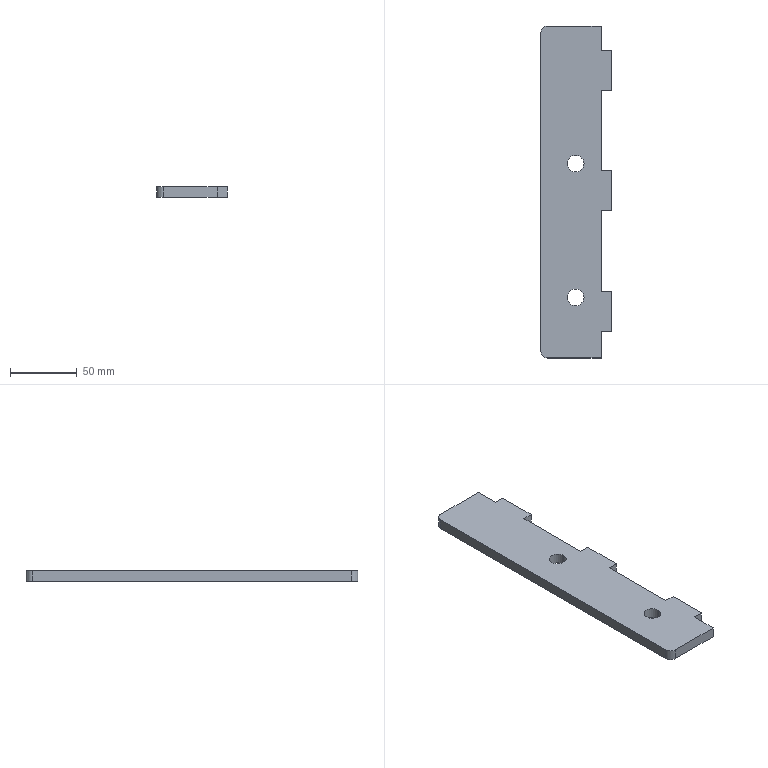Part | SolidWorks | features FlatPattern 1, SMBaseFlange 1, SheetMetal 1 | 1 solid | 24 faces | box 52.5 x 248 x 8 mm | volume 92631 mm3 | plane 18 | cylinder 6 | commonest cylinder face diameters 12.5 x4 10 x2
STEP:
#1=CARTESIAN_POINT('',(-25.25,44.,8.));
#2=VERTEX_POINT('',#1);
#3=CARTESIAN_POINT('',(-12.75,44.,8.));
#4=VERTEX_POINT('',#3);
#5=CARTESIAN_POINT('',(-19.,44.,8.));
#6=DIRECTION('',(0.,0.,1.));
#7=DIRECTION('',(1.,0.,0.));
#8=AXIS2_PLACEMENT_3D('',#5,#6,#7);
#9=CIRCLE('',#8,6.25);
#10=EDGE_CURVE('',#2,#4,#9,.T.);
#11=ORIENTED_EDGE('',*,*,#10,.T.);
#12=CARTESIAN_POINT('',(-12.75,44.,0.));
#13=VERTEX_POINT('',#12);
#14=CARTESIAN_POINT('',(-12.75,44.,8.));
#15=DIRECTION('',(0.,0.,-1.));
#16=VECTOR('',#15,1000.);
#17=LINE('',#14,#16);
#18=EDGE_CURVE('',#4,#13,#17,.T.);
#19=ORIENTED_EDGE('',*,*,#18,.T.);
#20=CARTESIAN_POINT('',(-25.25,44.,0.));
#21=VERTEX_POINT('',#20);
#22=CARTESIAN_POINT('',(-19.,44.,0.));
#23=DIRECTION('',(0.,0.,1.));
#24=DIRECTION('',(1.,0.,0.));
#25=AXIS2_PLACEMENT_3D('',#22,#23,#24);
#26=CIRCLE('',#25,6.25);
#27=EDGE_CURVE('',#21,#13,#26,.T.);
#28=ORIENTED_EDGE('',*,*,#27,.F.);
#29=CARTESIAN_POINT('',(-25.25,44.,8.));
#30=DIRECTION('',(0.,0.,-1.));
#31=VECTOR('',#30,1000.);
#32=LINE('',#29,#31);
#33=EDGE_CURVE('',#2,#21,#32,.T.);
#34=ORIENTED_EDGE('',*,*,#33,.F.);
#35=EDGE_LOOP('',(#11,#19,#28,#34));
#36=FACE_OUTER_BOUND('',#35,.T.);
#37=CARTESIAN_POINT('',(-19.,44.,8.));
#38=DIRECTION('',(0.,0.,-1.));
#39=DIRECTION('',(-1.,0.,0.));
#40=AXIS2_PLACEMENT_3D('',#37,#38,#39);
#41=CYLINDRICAL_SURFACE('',#40,6.25);
#42=ADVANCED_FACE('',(#36),#41,.F.);
#43=CARTESIAN_POINT('',(-25.25,-56.,8.));
#44=VERTEX_POINT('',#43);
#45=CARTESIAN_POINT('',(-12.75,-56.,8.));
#46=VERTEX_POINT('',#45);
#47=CARTESIAN_POINT('',(-19.,-56.,8.));
#48=DIRECTION('',(0.,0.,1.));
#49=DIRECTION('',(1.,0.,0.));
#50=AXIS2_PLACEMENT_3D('',#47,#48,#49);
#51=CIRCLE('',#50,6.25);
#52=EDGE_CURVE('',#44,#46,#51,.T.);
#53=ORIENTED_EDGE('',*,*,#52,.T.);
#54=CARTESIAN_POINT('',(-12.75,-56.,0.));
#55=VERTEX_POINT('',#54);
#56=CARTESIAN_POINT('',(-12.75,-56.,8.));
#57=DIRECTION('',(0.,0.,-1.));
#58=VECTOR('',#57,1000.);
#59=LINE('',#56,#58);
#60=EDGE_CURVE('',#46,#55,#59,.T.);
#61=ORIENTED_EDGE('',*,*,#60,.T.);
#62=CARTESIAN_POINT('',(-25.25,-56.,0.));
#63=VERTEX_POINT('',#62);
#64=CARTESIAN_POINT('',(-19.,-56.,0.));
#65=DIRECTION('',(0.,0.,1.));
#66=DIRECTION('',(1.,0.,0.));
#67=AXIS2_PLACEMENT_3D('',#64,#65,#66);
#68=CIRCLE('',#67,6.25);
#69=EDGE_CURVE('',#63,#55,#68,.T.);
#70=ORIENTED_EDGE('',*,*,#69,.F.);
#71=CARTESIAN_POINT('',(-25.25,-56.,8.));
#72=DIRECTION('',(0.,0.,-1.));
#73=VECTOR('',#72,1000.);
#74=LINE('',#71,#73);
#75=EDGE_CURVE('',#44,#63,#74,.T.);
#76=ORIENTED_EDGE('',*,*,#75,.F.);
#77=EDGE_LOOP('',(#53,#61,#70,#76));
#78=FACE_OUTER_BOUND('',#77,.T.);
#79=CARTESIAN_POINT('',(-19.,-56.,8.));
#80=DIRECTION('',(0.,0.,-1.));
#81=DIRECTION('',(-1.,0.,0.));
#82=AXIS2_PLACEMENT_3D('',#79,#80,#81);
#83=CYLINDRICAL_SURFACE('',#82,6.25);
#84=ADVANCED_FACE('',(#78),#83,.F.);
#85=CARTESIAN_POINT('',(0.,-101.22,8.));
#86=VERTEX_POINT('',#85);
#87=CARTESIAN_POINT('',(0.,-81.22,8.));
#88=VERTEX_POINT('',#87);
#89=CARTESIAN_POINT('',(0.,-101.22,8.));
#90=DIRECTION('',(0.,1.,0.));
#91=VECTOR('',#90,1000.);
#92=LINE('',#89,#91);
#93=EDGE_CURVE('',#86,#88,#92,.T.);
#94=ORIENTED_EDGE('',*,*,#93,.T.);
#95=CARTESIAN_POINT('',(7.5,-81.22,8.));
#96=VERTEX_POINT('',#95);
#97=CARTESIAN_POINT('',(0.,-81.22,8.));
#98=DIRECTION('',(1.,0.,0.));
#99=VECTOR('',#98,1000.);
#100=LINE('',#97,#99);
#101=EDGE_CURVE('',#88,#96,#100,.T.);
#102=ORIENTED_EDGE('',*,*,#101,.T.);
#103=CARTESIAN_POINT('',(7.5,-51.22,8.));
#104=VERTEX_POINT('',#103);
#105=CARTESIAN_POINT('',(7.5,-81.22,8.));
#106=DIRECTION('',(0.,1.,0.));
#107=VECTOR('',#106,1000.);
#108=LINE('',#105,#107);
#109=EDGE_CURVE('',#96,#104,#108,.T.);
#110=ORIENTED_EDGE('',*,*,#109,.T.);
#111=CARTESIAN_POINT('',(0.,-51.22,8.));
#112=VERTEX_POINT('',#111);
#113=CARTESIAN_POINT('',(7.5,-51.22,8.));
#114=DIRECTION('',(-1.,0.,0.));
#115=VECTOR('',#114,1000.);
#116=LINE('',#113,#115);
#117=EDGE_CURVE('',#104,#112,#116,.T.);
#118=ORIENTED_EDGE('',*,*,#117,.T.);
#119=CARTESIAN_POINT('',(0.,8.78,8.));
#120=VERTEX_POINT('',#119);
#121=CARTESIAN_POINT('',(0.,8.78,8.));
#122=DIRECTION('',(0.,1.,0.));
#123=VECTOR('',#122,1000.);
#124=LINE('',#121,#123);
#125=EDGE_CURVE('',#112,#120,#124,.T.);
#126=ORIENTED_EDGE('',*,*,#125,.T.);
#127=CARTESIAN_POINT('',(7.5,8.78,8.));
#128=VERTEX_POINT('',#127);
#129=CARTESIAN_POINT('',(0.,8.78,8.));
#130=DIRECTION('',(1.,0.,0.));
#131=VECTOR('',#130,1000.);
#132=LINE('',#129,#131);
#133=EDGE_CURVE('',#120,#128,#132,.T.);
#134=ORIENTED_EDGE('',*,*,#133,.T.);
#135=CARTESIAN_POINT('',(7.5,38.78,8.));
#136=VERTEX_POINT('',#135);
#137=CARTESIAN_POINT('',(7.5,8.78,8.));
#138=DIRECTION('',(0.,1.,0.));
#139=VECTOR('',#138,1000.);
#140=LINE('',#137,#139);
#141=EDGE_CURVE('',#128,#136,#140,.T.);
#142=ORIENTED_EDGE('',*,*,#141,.T.);
#143=CARTESIAN_POINT('',(0.,38.78,8.));
#144=VERTEX_POINT('',#143);
#145=CARTESIAN_POINT('',(7.5,38.78,8.));
#146=DIRECTION('',(-1.,0.,0.));
#147=VECTOR('',#146,1000.);
#148=LINE('',#145,#147);
#149=EDGE_CURVE('',#136,#144,#148,.T.);
#150=ORIENTED_EDGE('',*,*,#149,.T.);
#151=CARTESIAN_POINT('',(0.,98.78,8.));
#152=VERTEX_POINT('',#151);
#153=CARTESIAN_POINT('',(0.,98.78,8.));
#154=DIRECTION('',(0.,1.,0.));
#155=VECTOR('',#154,1000.);
#156=LINE('',#153,#155);
#157=EDGE_CURVE('',#144,#152,#156,.T.);
#158=ORIENTED_EDGE('',*,*,#157,.T.);
#159=CARTESIAN_POINT('',(7.5,98.78,8.));
#160=VERTEX_POINT('',#159);
#161=CARTESIAN_POINT('',(0.,98.78,8.));
#162=DIRECTION('',(1.,0.,0.));
#163=VECTOR('',#162,1000.);
#164=LINE('',#161,#163);
#165=EDGE_CURVE('',#152,#160,#164,.T.);
#166=ORIENTED_EDGE('',*,*,#165,.T.);
#167=CARTESIAN_POINT('',(7.5,128.78,8.));
#168=VERTEX_POINT('',#167);
#169=CARTESIAN_POINT('',(7.5,98.78,8.));
#170=DIRECTION('',(0.,1.,0.));
#171=VECTOR('',#170,1000.);
#172=LINE('',#169,#171);
#173=EDGE_CURVE('',#160,#168,#172,.T.);
#174=ORIENTED_EDGE('',*,*,#173,.T.);
#175=CARTESIAN_POINT('',(0.,128.78,8.));
#176=VERTEX_POINT('',#175);
#177=CARTESIAN_POINT('',(7.5,128.78,8.));
#178=DIRECTION('',(-1.,0.,0.));
#179=VECTOR('',#178,1000.);
#180=LINE('',#177,#179);
#181=EDGE_CURVE('',#168,#176,#180,.T.);
#182=ORIENTED_EDGE('',*,*,#181,.T.);
#183=CARTESIAN_POINT('',(0.,146.78,8.));
#184=VERTEX_POINT('',#183);
#185=CARTESIAN_POINT('',(0.,146.78,8.));
#186=DIRECTION('',(0.,1.,0.));
#187=VECTOR('',#186,1000.);
#188=LINE('',#185,#187);
#189=EDGE_CURVE('',#176,#184,#188,.T.);
#190=ORIENTED_EDGE('',*,*,#189,.T.);
#191=CARTESIAN_POINT('',(-40.,146.78,8.));
#192=VERTEX_POINT('',#191);
#193=CARTESIAN_POINT('',(-40.,146.78,8.));
#194=DIRECTION('',(-1.,0.,0.));
#195=VECTOR('',#194,1000.);
#196=LINE('',#193,#195);
#197=EDGE_CURVE('',#184,#192,#196,.T.);
#198=ORIENTED_EDGE('',*,*,#197,.T.);
#199=CARTESIAN_POINT('',(-45.,141.78,8.));
#200=VERTEX_POINT('',#199);
#201=CARTESIAN_POINT('',(-40.,141.78,8.));
#202=DIRECTION('',(0.,0.,1.));
#203=DIRECTION('',(-1.,0.,0.));
#204=AXIS2_PLACEMENT_3D('',#201,#202,#203);
#205=CIRCLE('',#204,5.);
#206=EDGE_CURVE('',#192,#200,#205,.T.);
#207=ORIENTED_EDGE('',*,*,#206,.T.);
#208=CARTESIAN_POINT('',(-45.,-96.22,8.));
#209=VERTEX_POINT('',#208);
#210=CARTESIAN_POINT('',(-45.,-96.22,8.));
#211=DIRECTION('',(0.,-1.,0.));
#212=VECTOR('',#211,1000.);
#213=LINE('',#210,#212);
#214=EDGE_CURVE('',#200,#209,#213,.T.);
#215=ORIENTED_EDGE('',*,*,#214,.T.);
#216=CARTESIAN_POINT('',(-40.,-101.22,8.));
#217=VERTEX_POINT('',#216);
#218=CARTESIAN_POINT('',(-40.,-96.22,8.));
#219=DIRECTION('',(0.,0.,1.));
#220=DIRECTION('',(-1.,0.,0.));
#221=AXIS2_PLACEMENT_3D('',#218,#219,#220);
#222=CIRCLE('',#221,5.);
#223=EDGE_CURVE('',#209,#217,#222,.T.);
#224=ORIENTED_EDGE('',*,*,#223,.T.);
#225=CARTESIAN_POINT('',(0.,-101.22,8.));
#226=DIRECTION('',(1.,0.,0.));
#227=VECTOR('',#226,1000.);
#228=LINE('',#225,#227);
#229=EDGE_CURVE('',#217,#86,#228,.T.);
#230=ORIENTED_EDGE('',*,*,#229,.T.);
#231=EDGE_LOOP('',(#94,#102,#110,#118,#126,#134,#142,#150,#158,#166,#174,#182,#190,#198,#207,#215,#224,#230));
#232=FACE_OUTER_BOUND('',#231,.T.);
#233=ORIENTED_EDGE('',*,*,#52,.F.);
#234=CARTESIAN_POINT('',(-19.,-56.,8.));
#235=DIRECTION('',(0.,0.,1.));
#236=DIRECTION('',(1.,0.,0.));
#237=AXIS2_PLACEMENT_3D('',#234,#235,#236);
#238=CIRCLE('',#237,6.25);
#239=EDGE_CURVE('',#46,#44,#238,.T.);
#240=ORIENTED_EDGE('',*,*,#239,.F.);
#241=EDGE_LOOP('',(#233,#240));
#242=FACE_BOUND('',#241,.T.);
#243=ORIENTED_EDGE('',*,*,#10,.F.);
#244=CARTESIAN_POINT('',(-19.,44.,8.));
#245=DIRECTION('',(0.,0.,1.));
#246=DIRECTION('',(1.,0.,0.));
#247=AXIS2_PLACEMENT_3D('',#244,#245,#246);
#248=CIRCLE('',#247,6.25);
#249=EDGE_CURVE('',#4,#2,#248,.T.);
#250=ORIENTED_EDGE('',*,*,#249,.F.);
#251=EDGE_LOOP('',(#243,#250));
#252=FACE_BOUND('',#251,.T.);
#253=CARTESIAN_POINT('',(-40.,141.78,8.));
#254=DIRECTION('',(0.,0.,-1.));
#255=DIRECTION('',(-1.,0.,0.));
#256=AXIS2_PLACEMENT_3D('',#253,#254,#255);
#257=PLANE('',#256);
#258=ADVANCED_FACE('',(#232,#242,#252),#257,.F.);
#259=ORIENTED_EDGE('',*,*,#69,.T.);
#260=CARTESIAN_POINT('',(-19.,-56.,0.));
#261=DIRECTION('',(0.,0.,1.));
#262=DIRECTION('',(1.,0.,0.));
#263=AXIS2_PLACEMENT_3D('',#260,#261,#262);
#264=CIRCLE('',#263,6.25);
#265=EDGE_CURVE('',#55,#63,#264,.T.);
#266=ORIENTED_EDGE('',*,*,#265,.T.);
#267=EDGE_LOOP('',(#259,#266));
#268=FACE_BOUND('',#267,.T.);
#269=CARTESIAN_POINT('',(0.,-101.22,0.));
#270=VERTEX_POINT('',#269);
#271=CARTESIAN_POINT('',(0.,-81.22,0.));
#272=VERTEX_POINT('',#271);
#273=CARTESIAN_POINT('',(0.,-101.22,0.));
#274=DIRECTION('',(0.,1.,0.));
#275=VECTOR('',#274,1000.);
#276=LINE('',#273,#275);
#277=EDGE_CURVE('',#270,#272,#276,.T.);
#278=ORIENTED_EDGE('',*,*,#277,.F.);
#279=CARTESIAN_POINT('',(-40.,-101.22,0.));
#280=VERTEX_POINT('',#279);
#281=CARTESIAN_POINT('',(0.,-101.22,0.));
#282=DIRECTION('',(1.,0.,0.));
#283=VECTOR('',#282,1000.);
#284=LINE('',#281,#283);
#285=EDGE_CURVE('',#280,#270,#284,.T.);
#286=ORIENTED_EDGE('',*,*,#285,.F.);
#287=CARTESIAN_POINT('',(-45.,-96.22,0.));
#288=VERTEX_POINT('',#287);
#289=CARTESIAN_POINT('',(-40.,-96.22,0.));
#290=DIRECTION('',(0.,0.,1.));
#291=DIRECTION('',(-1.,0.,0.));
#292=AXIS2_PLACEMENT_3D('',#289,#290,#291);
#293=CIRCLE('',#292,5.);
#294=EDGE_CURVE('',#288,#280,#293,.T.);
#295=ORIENTED_EDGE('',*,*,#294,.F.);
#296=CARTESIAN_POINT('',(-45.,141.78,0.));
#297=VERTEX_POINT('',#296);
#298=CARTESIAN_POINT('',(-45.,-96.22,0.));
#299=DIRECTION('',(0.,-1.,0.));
#300=VECTOR('',#299,1000.);
#301=LINE('',#298,#300);
#302=EDGE_CURVE('',#297,#288,#301,.T.);
#303=ORIENTED_EDGE('',*,*,#302,.F.);
#304=CARTESIAN_POINT('',(-40.,146.78,0.));
#305=VERTEX_POINT('',#304);
#306=CARTESIAN_POINT('',(-40.,141.78,0.));
#307=DIRECTION('',(0.,0.,1.));
#308=DIRECTION('',(-1.,0.,0.));
#309=AXIS2_PLACEMENT_3D('',#306,#307,#308);
#310=CIRCLE('',#309,5.);
#311=EDGE_CURVE('',#305,#297,#310,.T.);
#312=ORIENTED_EDGE('',*,*,#311,.F.);
#313=CARTESIAN_POINT('',(0.,146.78,0.));
#314=VERTEX_POINT('',#313);
#315=CARTESIAN_POINT('',(-40.,146.78,0.));
#316=DIRECTION('',(-1.,0.,0.));
#317=VECTOR('',#316,1000.);
#318=LINE('',#315,#317);
#319=EDGE_CURVE('',#314,#305,#318,.T.);
#320=ORIENTED_EDGE('',*,*,#319,.F.);
#321=CARTESIAN_POINT('',(0.,128.78,0.));
#322=VERTEX_POINT('',#321);
#323=CARTESIAN_POINT('',(0.,146.78,0.));
#324=DIRECTION('',(0.,1.,0.));
#325=VECTOR('',#324,1000.);
#326=LINE('',#323,#325);
#327=EDGE_CURVE('',#322,#314,#326,.T.);
#328=ORIENTED_EDGE('',*,*,#327,.F.);
#329=CARTESIAN_POINT('',(7.5,128.78,0.));
#330=VERTEX_POINT('',#329);
#331=CARTESIAN_POINT('',(7.5,128.78,0.));
#332=DIRECTION('',(-1.,0.,0.));
#333=VECTOR('',#332,1000.);
#334=LINE('',#331,#333);
#335=EDGE_CURVE('',#330,#322,#334,.T.);
#336=ORIENTED_EDGE('',*,*,#335,.F.);
#337=CARTESIAN_POINT('',(7.5,98.78,0.));
#338=VERTEX_POINT('',#337);
#339=CARTESIAN_POINT('',(7.5,98.78,0.));
#340=DIRECTION('',(0.,1.,0.));
#341=VECTOR('',#340,1000.);
#342=LINE('',#339,#341);
#343=EDGE_CURVE('',#338,#330,#342,.T.);
#344=ORIENTED_EDGE('',*,*,#343,.F.);
#345=CARTESIAN_POINT('',(0.,98.78,0.));
#346=VERTEX_POINT('',#345);
#347=CARTESIAN_POINT('',(0.,98.78,0.));
#348=DIRECTION('',(1.,0.,0.));
#349=VECTOR('',#348,1000.);
#350=LINE('',#347,#349);
#351=EDGE_CURVE('',#346,#338,#350,.T.);
#352=ORIENTED_EDGE('',*,*,#351,.F.);
#353=CARTESIAN_POINT('',(0.,38.78,0.));
#354=VERTEX_POINT('',#353);
#355=CARTESIAN_POINT('',(0.,98.78,0.));
#356=DIRECTION('',(0.,1.,0.));
#357=VECTOR('',#356,1000.);
#358=LINE('',#355,#357);
#359=EDGE_CURVE('',#354,#346,#358,.T.);
#360=ORIENTED_EDGE('',*,*,#359,.F.);
#361=CARTESIAN_POINT('',(7.5,38.78,0.));
#362=VERTEX_POINT('',#361);
#363=CARTESIAN_POINT('',(7.5,38.78,0.));
#364=DIRECTION('',(-1.,0.,0.));
#365=VECTOR('',#364,1000.);
#366=LINE('',#363,#365);
#367=EDGE_CURVE('',#362,#354,#366,.T.);
#368=ORIENTED_EDGE('',*,*,#367,.F.);
#369=CARTESIAN_POINT('',(7.5,8.78,0.));
#370=VERTEX_POINT('',#369);
#371=CARTESIAN_POINT('',(7.5,8.78,0.));
#372=DIRECTION('',(0.,1.,0.));
#373=VECTOR('',#372,1000.);
#374=LINE('',#371,#373);
#375=EDGE_CURVE('',#370,#362,#374,.T.);
#376=ORIENTED_EDGE('',*,*,#375,.F.);
#377=CARTESIAN_POINT('',(0.,8.78,0.));
#378=VERTEX_POINT('',#377);
#379=CARTESIAN_POINT('',(0.,8.78,0.));
#380=DIRECTION('',(1.,0.,0.));
#381=VECTOR('',#380,1000.);
#382=LINE('',#379,#381);
#383=EDGE_CURVE('',#378,#370,#382,.T.);
#384=ORIENTED_EDGE('',*,*,#383,.F.);
#385=CARTESIAN_POINT('',(0.,-51.22,0.));
#386=VERTEX_POINT('',#385);
#387=CARTESIAN_POINT('',(0.,8.78,0.));
#388=DIRECTION('',(0.,1.,0.));
#389=VECTOR('',#388,1000.);
#390=LINE('',#387,#389);
#391=EDGE_CURVE('',#386,#378,#390,.T.);
#392=ORIENTED_EDGE('',*,*,#391,.F.);
#393=CARTESIAN_POINT('',(7.5,-51.22,0.));
#394=VERTEX_POINT('',#393);
#395=CARTESIAN_POINT('',(7.5,-51.22,0.));
#396=DIRECTION('',(-1.,0.,0.));
#397=VECTOR('',#396,1000.);
#398=LINE('',#395,#397);
#399=EDGE_CURVE('',#394,#386,#398,.T.);
#400=ORIENTED_EDGE('',*,*,#399,.F.);
#401=CARTESIAN_POINT('',(7.5,-81.22,0.));
#402=VERTEX_POINT('',#401);
#403=CARTESIAN_POINT('',(7.5,-81.22,0.));
#404=DIRECTION('',(0.,1.,0.));
#405=VECTOR('',#404,1000.);
#406=LINE('',#403,#405);
#407=EDGE_CURVE('',#402,#394,#406,.T.);
#408=ORIENTED_EDGE('',*,*,#407,.F.);
#409=CARTESIAN_POINT('',(0.,-81.22,0.));
#410=DIRECTION('',(1.,0.,0.));
#411=VECTOR('',#410,1000.);
#412=LINE('',#409,#411);
#413=EDGE_CURVE('',#272,#402,#412,.T.);
#414=ORIENTED_EDGE('',*,*,#413,.F.);
#415=EDGE_LOOP('',(#278,#286,#295,#303,#312,#320,#328,#336,#344,#352,#360,#368,#376,#384,#392,#400,#408,#414));
#416=FACE_OUTER_BOUND('',#415,.T.);
#417=ORIENTED_EDGE('',*,*,#27,.T.);
#418=CARTESIAN_POINT('',(-19.,44.,0.));
#419=DIRECTION('',(0.,0.,1.));
#420=DIRECTION('',(1.,0.,0.));
#421=AXIS2_PLACEMENT_3D('',#418,#419,#420);
#422=CIRCLE('',#421,6.25);
#423=EDGE_CURVE('',#13,#21,#422,.T.);
#424=ORIENTED_EDGE('',*,*,#423,.T.);
#425=EDGE_LOOP('',(#417,#424));
#426=FACE_BOUND('',#425,.T.);
#427=CARTESIAN_POINT('',(-40.,141.78,0.));
#428=DIRECTION('',(0.,0.,-1.));
#429=DIRECTION('',(-1.,0.,0.));
#430=AXIS2_PLACEMENT_3D('',#427,#428,#429);
#431=PLANE('',#430);
#432=ADVANCED_FACE('',(#268,#416,#426),#431,.T.);
#433=ORIENTED_EDGE('',*,*,#277,.T.);
#434=CARTESIAN_POINT('',(0.,-81.22,8.));
#435=DIRECTION('',(0.,0.,-1.));
#436=VECTOR('',#435,1000.);
#437=LINE('',#434,#436);
#438=EDGE_CURVE('',#88,#272,#437,.T.);
#439=ORIENTED_EDGE('',*,*,#438,.F.);
#440=ORIENTED_EDGE('',*,*,#93,.F.);
#441=CARTESIAN_POINT('',(0.,-101.22,8.));
#442=DIRECTION('',(0.,0.,-1.));
#443=VECTOR('',#442,1000.);
#444=LINE('',#441,#443);
#445=EDGE_CURVE('',#86,#270,#444,.T.);
#446=ORIENTED_EDGE('',*,*,#445,.T.);
#447=EDGE_LOOP('',(#433,#439,#440,#446));
#448=FACE_OUTER_BOUND('',#447,.T.);
#449=CARTESIAN_POINT('',(0.,-101.22,8.));
#450=DIRECTION('',(-1.,0.,0.));
#451=DIRECTION('',(0.,-1.,0.));
#452=AXIS2_PLACEMENT_3D('',#449,#450,#451);
#453=PLANE('',#452);
#454=ADVANCED_FACE('',(#448),#453,.F.);
#455=ORIENTED_EDGE('',*,*,#413,.T.);
#456=CARTESIAN_POINT('',(7.5,-81.22,8.));
#457=DIRECTION('',(0.,0.,-1.));
#458=VECTOR('',#457,1000.);
#459=LINE('',#456,#458);
#460=EDGE_CURVE('',#96,#402,#459,.T.);
#461=ORIENTED_EDGE('',*,*,#460,.F.);
#462=ORIENTED_EDGE('',*,*,#101,.F.);
#463=ORIENTED_EDGE('',*,*,#438,.T.);
#464=EDGE_LOOP('',(#455,#461,#462,#463));
#465=FACE_OUTER_BOUND('',#464,.T.);
#466=CARTESIAN_POINT('',(0.,-81.22,8.));
#467=DIRECTION('',(0.,1.,0.));
#468=DIRECTION('',(0.,0.,1.));
#469=AXIS2_PLACEMENT_3D('',#466,#467,#468);
#470=PLANE('',#469);
#471=ADVANCED_FACE('',(#465),#470,.F.);
#472=ORIENTED_EDGE('',*,*,#407,.T.);
#473=CARTESIAN_POINT('',(7.5,-51.22,8.));
#474=DIRECTION('',(0.,0.,-1.));
#475=VECTOR('',#474,1000.);
#476=LINE('',#473,#475);
#477=EDGE_CURVE('',#104,#394,#476,.T.);
#478=ORIENTED_EDGE('',*,*,#477,.F.);
#479=ORIENTED_EDGE('',*,*,#109,.F.);
#480=ORIENTED_EDGE('',*,*,#460,.T.);
#481=EDGE_LOOP('',(#472,#478,#479,#480));
#482=FACE_OUTER_BOUND('',#481,.T.);
#483=CARTESIAN_POINT('',(7.5,-81.22,8.));
#484=DIRECTION('',(-1.,0.,0.));
#485=DIRECTION('',(0.,0.,1.));
#486=AXIS2_PLACEMENT_3D('',#483,#484,#485);
#487=PLANE('',#486);
#488=ADVANCED_FACE('',(#482),#487,.F.);
#489=ORIENTED_EDGE('',*,*,#399,.T.);
#490=CARTESIAN_POINT('',(0.,-51.22,8.));
#491=DIRECTION('',(0.,0.,-1.));
#492=VECTOR('',#491,1000.);
#493=LINE('',#490,#492);
#494=EDGE_CURVE('',#112,#386,#493,.T.);
#495=ORIENTED_EDGE('',*,*,#494,.F.);
#496=ORIENTED_EDGE('',*,*,#117,.F.);
#497=ORIENTED_EDGE('',*,*,#477,.T.);
#498=EDGE_LOOP('',(#489,#495,#496,#497));
#499=FACE_OUTER_BOUND('',#498,.T.);
#500=CARTESIAN_POINT('',(7.5,-51.22,8.));
#501=DIRECTION('',(0.,-1.,0.));
#502=DIRECTION('',(0.,0.,-1.));
#503=AXIS2_PLACEMENT_3D('',#500,#501,#502);
#504=PLANE('',#503);
#505=ADVANCED_FACE('',(#499),#504,.F.);
#506=ORIENTED_EDGE('',*,*,#391,.T.);
#507=CARTESIAN_POINT('',(0.,8.78,8.));
#508=DIRECTION('',(0.,0.,-1.));
#509=VECTOR('',#508,1000.);
#510=LINE('',#507,#509);
#511=EDGE_CURVE('',#120,#378,#510,.T.);
#512=ORIENTED_EDGE('',*,*,#511,.F.);
#513=ORIENTED_EDGE('',*,*,#125,.F.);
#514=ORIENTED_EDGE('',*,*,#494,.T.);
#515=EDGE_LOOP('',(#506,#512,#513,#514));
#516=FACE_OUTER_BOUND('',#515,.T.);
#517=CARTESIAN_POINT('',(0.,8.78,8.));
#518=DIRECTION('',(-1.,0.,0.));
#519=DIRECTION('',(0.,-1.,0.));
#520=AXIS2_PLACEMENT_3D('',#517,#518,#519);
#521=PLANE('',#520);
#522=ADVANCED_FACE('',(#516),#521,.F.);
#523=ORIENTED_EDGE('',*,*,#383,.T.);
#524=CARTESIAN_POINT('',(7.5,8.78,8.));
#525=DIRECTION('',(0.,0.,-1.));
#526=VECTOR('',#525,1000.);
#527=LINE('',#524,#526);
#528=EDGE_CURVE('',#128,#370,#527,.T.);
#529=ORIENTED_EDGE('',*,*,#528,.F.);
#530=ORIENTED_EDGE('',*,*,#133,.F.);
#531=ORIENTED_EDGE('',*,*,#511,.T.);
#532=EDGE_LOOP('',(#523,#529,#530,#531));
#533=FACE_OUTER_BOUND('',#532,.T.);
#534=CARTESIAN_POINT('',(0.,8.78,8.));
#535=DIRECTION('',(0.,1.,0.));
#536=DIRECTION('',(0.,0.,1.));
#537=AXIS2_PLACEMENT_3D('',#534,#535,#536);
#538=PLANE('',#537);
#539=ADVANCED_FACE('',(#533),#538,.F.);
#540=ORIENTED_EDGE('',*,*,#375,.T.);
#541=CARTESIAN_POINT('',(7.5,38.78,8.));
#542=DIRECTION('',(0.,0.,-1.));
#543=VECTOR('',#542,1000.);
#544=LINE('',#541,#543);
#545=EDGE_CURVE('',#136,#362,#544,.T.);
#546=ORIENTED_EDGE('',*,*,#545,.F.);
#547=ORIENTED_EDGE('',*,*,#141,.F.);
#548=ORIENTED_EDGE('',*,*,#528,.T.);
#549=EDGE_LOOP('',(#540,#546,#547,#548));
#550=FACE_OUTER_BOUND('',#549,.T.);
#551=CARTESIAN_POINT('',(7.5,8.78,8.));
#552=DIRECTION('',(-1.,0.,0.));
#553=DIRECTION('',(0.,-1.,0.));
#554=AXIS2_PLACEMENT_3D('',#551,#552,#553);
#555=PLANE('',#554);
#556=ADVANCED_FACE('',(#550),#555,.F.);
#557=ORIENTED_EDGE('',*,*,#367,.T.);
#558=CARTESIAN_POINT('',(0.,38.78,8.));
#559=DIRECTION('',(0.,0.,-1.));
#560=VECTOR('',#559,1000.);
#561=LINE('',#558,#560);
#562=EDGE_CURVE('',#144,#354,#561,.T.);
#563=ORIENTED_EDGE('',*,*,#562,.F.);
#564=ORIENTED_EDGE('',*,*,#149,.F.);
#565=ORIENTED_EDGE('',*,*,#545,.T.);
#566=EDGE_LOOP('',(#557,#563,#564,#565));
#567=FACE_OUTER_BOUND('',#566,.T.);
#568=CARTESIAN_POINT('',(7.5,38.78,8.));
#569=DIRECTION('',(0.,-1.,0.));
#570=DIRECTION('',(0.,0.,-1.));
#571=AXIS2_PLACEMENT_3D('',#568,#569,#570);
#572=PLANE('',#571);
#573=ADVANCED_FACE('',(#567),#572,.F.);
#574=ORIENTED_EDGE('',*,*,#359,.T.);
#575=CARTESIAN_POINT('',(0.,98.78,8.));
#576=DIRECTION('',(0.,0.,-1.));
#577=VECTOR('',#576,1000.);
#578=LINE('',#575,#577);
#579=EDGE_CURVE('',#152,#346,#578,.T.);
#580=ORIENTED_EDGE('',*,*,#579,.F.);
#581=ORIENTED_EDGE('',*,*,#157,.F.);
#582=ORIENTED_EDGE('',*,*,#562,.T.);
#583=EDGE_LOOP('',(#574,#580,#581,#582));
#584=FACE_OUTER_BOUND('',#583,.T.);
#585=CARTESIAN_POINT('',(0.,98.78,8.));
#586=DIRECTION('',(-1.,0.,0.));
#587=DIRECTION('',(0.,-1.,0.));
#588=AXIS2_PLACEMENT_3D('',#585,#586,#587);
#589=PLANE('',#588);
#590=ADVANCED_FACE('',(#584),#589,.F.);
#591=ORIENTED_EDGE('',*,*,#351,.T.);
#592=CARTESIAN_POINT('',(7.5,98.78,8.));
#593=DIRECTION('',(0.,0.,-1.));
#594=VECTOR('',#593,1000.);
#595=LINE('',#592,#594);
#596=EDGE_CURVE('',#160,#338,#595,.T.);
#597=ORIENTED_EDGE('',*,*,#596,.F.);
#598=ORIENTED_EDGE('',*,*,#165,.F.);
#599=ORIENTED_EDGE('',*,*,#579,.T.);
#600=EDGE_LOOP('',(#591,#597,#598,#599));
#601=FACE_OUTER_BOUND('',#600,.T.);
#602=CARTESIAN_POINT('',(0.,98.78,8.));
#603=DIRECTION('',(0.,1.,0.));
#604=DIRECTION('',(0.,0.,1.));
#605=AXIS2_PLACEMENT_3D('',#602,#603,#604);
#606=PLANE('',#605);
#607=ADVANCED_FACE('',(#601),#606,.F.);
#608=ORIENTED_EDGE('',*,*,#343,.T.);
#609=CARTESIAN_POINT('',(7.5,128.78,8.));
#610=DIRECTION('',(0.,0.,-1.));
#611=VECTOR('',#610,1000.);
#612=LINE('',#609,#611);
#613=EDGE_CURVE('',#168,#330,#612,.T.);
#614=ORIENTED_EDGE('',*,*,#613,.F.);
#615=ORIENTED_EDGE('',*,*,#173,.F.);
#616=ORIENTED_EDGE('',*,*,#596,.T.);
#617=EDGE_LOOP('',(#608,#614,#615,#616));
#618=FACE_OUTER_BOUND('',#617,.T.);
#619=CARTESIAN_POINT('',(7.5,98.78,8.));
#620=DIRECTION('',(-1.,0.,0.));
#621=DIRECTION('',(0.,0.,1.));
#622=AXIS2_PLACEMENT_3D('',#619,#620,#621);
#623=PLANE('',#622);
#624=ADVANCED_FACE('',(#618),#623,.F.);
#625=ORIENTED_EDGE('',*,*,#335,.T.);
#626=CARTESIAN_POINT('',(0.,128.78,8.));
#627=DIRECTION('',(0.,0.,-1.));
#628=VECTOR('',#627,1000.);
#629=LINE('',#626,#628);
#630=EDGE_CURVE('',#176,#322,#629,.T.);
#631=ORIENTED_EDGE('',*,*,#630,.F.);
#632=ORIENTED_EDGE('',*,*,#181,.F.);
#633=ORIENTED_EDGE('',*,*,#613,.T.);
#634=EDGE_LOOP('',(#625,#631,#632,#633));
#635=FACE_OUTER_BOUND('',#634,.T.);
#636=CARTESIAN_POINT('',(7.5,128.78,8.));
#637=DIRECTION('',(0.,-1.,0.));
#638=DIRECTION('',(0.,0.,-1.));
#639=AXIS2_PLACEMENT_3D('',#636,#637,#638);
#640=PLANE('',#639);
#641=ADVANCED_FACE('',(#635),#640,.F.);
#642=ORIENTED_EDGE('',*,*,#327,.T.);
#643=CARTESIAN_POINT('',(0.,146.78,8.));
#644=DIRECTION('',(0.,0.,-1.));
#645=VECTOR('',#644,1000.);
#646=LINE('',#643,#645);
#647=EDGE_CURVE('',#184,#314,#646,.T.);
#648=ORIENTED_EDGE('',*,*,#647,.F.);
#649=ORIENTED_EDGE('',*,*,#189,.F.);
#650=ORIENTED_EDGE('',*,*,#630,.T.);
#651=EDGE_LOOP('',(#642,#648,#649,#650));
#652=FACE_OUTER_BOUND('',#651,.T.);
#653=CARTESIAN_POINT('',(0.,146.78,8.));
#654=DIRECTION('',(-1.,0.,0.));
#655=DIRECTION('',(0.,-1.,0.));
#656=AXIS2_PLACEMENT_3D('',#653,#654,#655);
#657=PLANE('',#656);
#658=ADVANCED_FACE('',(#652),#657,.F.);
#659=ORIENTED_EDGE('',*,*,#319,.T.);
#660=CARTESIAN_POINT('',(-40.,146.78,8.));
#661=DIRECTION('',(0.,0.,-1.));
#662=VECTOR('',#661,1000.);
#663=LINE('',#660,#662);
#664=EDGE_CURVE('',#192,#305,#663,.T.);
#665=ORIENTED_EDGE('',*,*,#664,.F.);
#666=ORIENTED_EDGE('',*,*,#197,.F.);
#667=ORIENTED_EDGE('',*,*,#647,.T.);
#668=EDGE_LOOP('',(#659,#665,#666,#667));
#669=FACE_OUTER_BOUND('',#668,.T.);
#670=CARTESIAN_POINT('',(-40.,146.78,8.));
#671=DIRECTION('',(0.,-1.,0.));
#672=DIRECTION('',(0.,0.,-1.));
#673=AXIS2_PLACEMENT_3D('',#670,#671,#672);
#674=PLANE('',#673);
#675=ADVANCED_FACE('',(#669),#674,.F.);
#676=ORIENTED_EDGE('',*,*,#311,.T.);
#677=CARTESIAN_POINT('',(-45.,141.78,8.));
#678=DIRECTION('',(0.,0.,-1.));
#679=VECTOR('',#678,1000.);
#680=LINE('',#677,#679);
#681=EDGE_CURVE('',#200,#297,#680,.T.);
#682=ORIENTED_EDGE('',*,*,#681,.F.);
#683=ORIENTED_EDGE('',*,*,#206,.F.);
#684=ORIENTED_EDGE('',*,*,#664,.T.);
#685=EDGE_LOOP('',(#676,#682,#683,#684));
#686=FACE_OUTER_BOUND('',#685,.T.);
#687=CARTESIAN_POINT('',(-40.,141.78,8.));
#688=DIRECTION('',(0.,0.,-1.));
#689=DIRECTION('',(-1.,0.,0.));
#690=AXIS2_PLACEMENT_3D('',#687,#688,#689);
#691=CYLINDRICAL_SURFACE('',#690,5.);
#692=ADVANCED_FACE('',(#686),#691,.T.);
#693=ORIENTED_EDGE('',*,*,#302,.T.);
#694=CARTESIAN_POINT('',(-45.,-96.22,8.));
#695=DIRECTION('',(0.,0.,-1.));
#696=VECTOR('',#695,1000.);
#697=LINE('',#694,#696);
#698=EDGE_CURVE('',#209,#288,#697,.T.);
#699=ORIENTED_EDGE('',*,*,#698,.F.);
#700=ORIENTED_EDGE('',*,*,#214,.F.);
#701=ORIENTED_EDGE('',*,*,#681,.T.);
#702=EDGE_LOOP('',(#693,#699,#700,#701));
#703=FACE_OUTER_BOUND('',#702,.T.);
#704=CARTESIAN_POINT('',(-45.,-96.22,8.));
#705=DIRECTION('',(1.,0.,0.));
#706=DIRECTION('',(0.,0.,-1.));
#707=AXIS2_PLACEMENT_3D('',#704,#705,#706);
#708=PLANE('',#707);
#709=ADVANCED_FACE('',(#703),#708,.F.);
#710=ORIENTED_EDGE('',*,*,#294,.T.);
#711=CARTESIAN_POINT('',(-40.,-101.22,8.));
#712=DIRECTION('',(0.,0.,-1.));
#713=VECTOR('',#712,1000.);
#714=LINE('',#711,#713);
#715=EDGE_CURVE('',#217,#280,#714,.T.);
#716=ORIENTED_EDGE('',*,*,#715,.F.);
#717=ORIENTED_EDGE('',*,*,#223,.F.);
#718=ORIENTED_EDGE('',*,*,#698,.T.);
#719=EDGE_LOOP('',(#710,#716,#717,#718));
#720=FACE_OUTER_BOUND('',#719,.T.);
#721=CARTESIAN_POINT('',(-40.,-96.22,8.));
#722=DIRECTION('',(0.,0.,-1.));
#723=DIRECTION('',(-1.,0.,0.));
#724=AXIS2_PLACEMENT_3D('',#721,#722,#723);
#725=CYLINDRICAL_SURFACE('',#724,5.);
#726=ADVANCED_FACE('',(#720),#725,.T.);
#727=ORIENTED_EDGE('',*,*,#285,.T.);
#728=ORIENTED_EDGE('',*,*,#445,.F.);
#729=ORIENTED_EDGE('',*,*,#229,.F.);
#730=ORIENTED_EDGE('',*,*,#715,.T.);
#731=EDGE_LOOP('',(#727,#728,#729,#730));
#732=FACE_OUTER_BOUND('',#731,.T.);
#733=CARTESIAN_POINT('',(0.,-101.22,8.));
#734=DIRECTION('',(0.,1.,0.));
#735=DIRECTION('',(0.,0.,1.));
#736=AXIS2_PLACEMENT_3D('',#733,#734,#735);
#737=PLANE('',#736);
#738=ADVANCED_FACE('',(#732),#737,.F.);
#739=ORIENTED_EDGE('',*,*,#60,.F.);
#740=ORIENTED_EDGE('',*,*,#239,.T.);
#741=ORIENTED_EDGE('',*,*,#75,.T.);
#742=ORIENTED_EDGE('',*,*,#265,.F.);
#743=EDGE_LOOP('',(#739,#740,#741,#742));
#744=FACE_OUTER_BOUND('',#743,.T.);
#745=CARTESIAN_POINT('',(-19.,-56.,8.));
#746=DIRECTION('',(0.,0.,-1.));
#747=DIRECTION('',(-1.,0.,0.));
#748=AXIS2_PLACEMENT_3D('',#745,#746,#747);
#749=CYLINDRICAL_SURFACE('',#748,6.25);
#750=ADVANCED_FACE('',(#744),#749,.F.);
#751=ORIENTED_EDGE('',*,*,#18,.F.);
#752=ORIENTED_EDGE('',*,*,#249,.T.);
#753=ORIENTED_EDGE('',*,*,#33,.T.);
#754=ORIENTED_EDGE('',*,*,#423,.F.);
#755=EDGE_LOOP('',(#751,#752,#753,#754));
#756=FACE_OUTER_BOUND('',#755,.T.);
#757=CARTESIAN_POINT('',(-19.,44.,8.));
#758=DIRECTION('',(0.,0.,-1.));
#759=DIRECTION('',(-1.,0.,0.));
#760=AXIS2_PLACEMENT_3D('',#757,#758,#759);
#761=CYLINDRICAL_SURFACE('',#760,6.25);
#762=ADVANCED_FACE('',(#756),#761,.F.);
#763=CLOSED_SHELL('',(#42,#84,#258,#432,#454,#471,#488,#505,#522,#539,#556,#573,#590,#607,#624,#641,#658,#675,#692,#709,#726,#738,#750,#762));
#764=MANIFOLD_SOLID_BREP('',#763);
#765=CARTESIAN_POINT('',(0.,0.,0.));
#766=DIRECTION('',(0.,0.,1.));
#767=DIRECTION('',(1.,0.,0.));
#768=AXIS2_PLACEMENT_3D('',#765,#766,#767);
#769=(LENGTH_UNIT()NAMED_UNIT(*)SI_UNIT(.MILLI.,.METRE.));
#770=UNCERTAINTY_MEASURE_WITH_UNIT(LENGTH_MEASURE(0.00001),#769,'','');
#771=(NAMED_UNIT(*)PLANE_ANGLE_UNIT()SI_UNIT($,.RADIAN.));
#772=(NAMED_UNIT(*)SI_UNIT($,.STERADIAN.)SOLID_ANGLE_UNIT());
#773=(GEOMETRIC_REPRESENTATION_CONTEXT(3)GLOBAL_UNCERTAINTY_ASSIGNED_CONTEXT((#770))GLOBAL_UNIT_ASSIGNED_CONTEXT((#769,#771,#772))REPRESENTATION_CONTEXT('',''));
#774=ADVANCED_BREP_SHAPE_REPRESENTATION('',(#764,#768),#773);